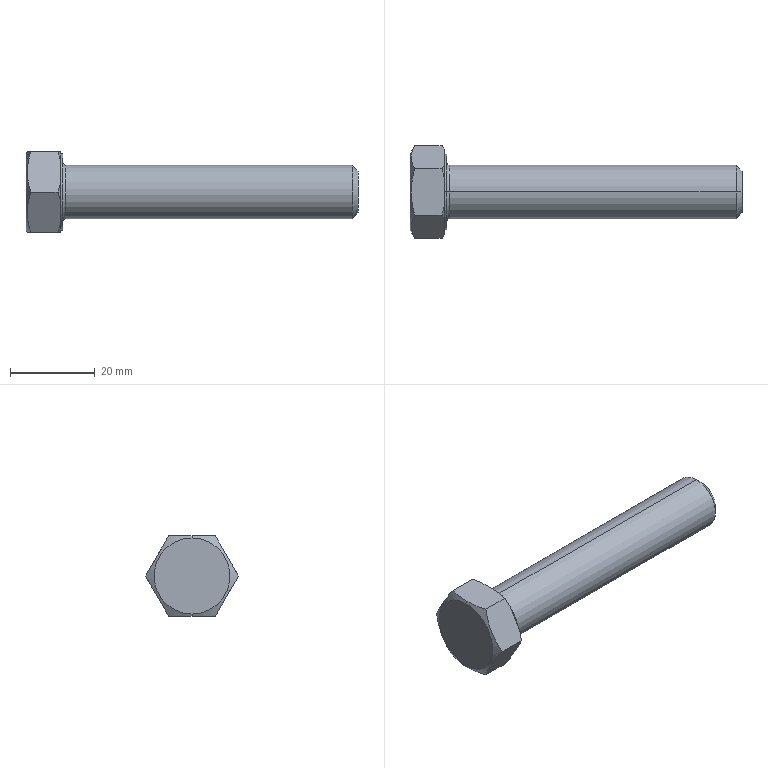Part | SolidWorks | features RevCut 4, Chamfer 1, Extrusion 1, Fillet 1, LPattern 1, Revolution 1 | 1 solid | 26 faces | box 78.581 x 21.997 x 19.05 mm | volume 11501 mm3 | cone 10 | plane 10 | cylinder 4 | torus 2 | commonest cylinder face diameters 12.7 x2 18 x2
STEP:
#1=CARTESIAN_POINT('',(9.331,0.,6.35));
#2=VERTEX_POINT('',#1);
#3=CARTESIAN_POINT('',(9.331,0.,-6.35));
#4=VERTEX_POINT('',#3);
#5=CARTESIAN_POINT('',(9.331,0.,0.));
#6=DIRECTION('',(1.,0.,0.));
#7=DIRECTION('',(0.,0.,-1.));
#8=AXIS2_PLACEMENT_3D('',#5,#6,#7);
#9=CIRCLE('',#8,6.35);
#10=EDGE_CURVE('',#2,#4,#9,.T.);
#11=ORIENTED_EDGE('',*,*,#10,.F.);
#12=CARTESIAN_POINT('',(8.731,0.,6.95));
#13=VERTEX_POINT('',#12);
#14=CARTESIAN_POINT('',(9.331,0.,6.95));
#15=DIRECTION('',(0.,1.,0.));
#16=DIRECTION('',(0.,0.,1.));
#17=AXIS2_PLACEMENT_3D('',#14,#15,#16);
#18=CIRCLE('',#17,0.6);
#19=EDGE_CURVE('',#2,#13,#18,.T.);
#20=ORIENTED_EDGE('',*,*,#19,.T.);
#21=CARTESIAN_POINT('',(8.731,0.,-6.95));
#22=VERTEX_POINT('',#21);
#23=CARTESIAN_POINT('',(8.731,0.,0.));
#24=DIRECTION('',(-1.,0.,0.));
#25=DIRECTION('',(0.,0.,-1.));
#26=AXIS2_PLACEMENT_3D('',#23,#24,#25);
#27=CIRCLE('',#26,6.95);
#28=EDGE_CURVE('',#22,#13,#27,.T.);
#29=ORIENTED_EDGE('',*,*,#28,.F.);
#30=CARTESIAN_POINT('',(9.331,0.,-6.95));
#31=DIRECTION('',(0.,-1.,0.));
#32=DIRECTION('',(0.,0.,-1.));
#33=AXIS2_PLACEMENT_3D('',#30,#31,#32);
#34=CIRCLE('',#33,0.6);
#35=EDGE_CURVE('',#4,#22,#34,.T.);
#36=ORIENTED_EDGE('',*,*,#35,.F.);
#37=EDGE_LOOP('',(#11,#20,#29,#36));
#38=FACE_OUTER_BOUND('',#37,.T.);
#39=CARTESIAN_POINT('',(9.331,0.,0.));
#40=DIRECTION('',(1.,0.,0.));
#41=DIRECTION('',(0.,0.,-1.));
#42=AXIS2_PLACEMENT_3D('',#39,#40,#41);
#43=TOROIDAL_SURFACE('',#42,6.95,0.6);
#44=ADVANCED_FACE('',(#38),#43,.F.);
#45=CARTESIAN_POINT('',(78.581,0.,-4.95));
#46=VERTEX_POINT('',#45);
#47=CARTESIAN_POINT('',(78.581,0.,4.95));
#48=VERTEX_POINT('',#47);
#49=CARTESIAN_POINT('',(78.581,0.,0.));
#50=DIRECTION('',(1.,0.,0.));
#51=DIRECTION('',(0.,0.,1.));
#52=AXIS2_PLACEMENT_3D('',#49,#50,#51);
#53=CIRCLE('',#52,4.95);
#54=EDGE_CURVE('',#46,#48,#53,.T.);
#55=ORIENTED_EDGE('',*,*,#54,.F.);
#56=CARTESIAN_POINT('',(77.181,0.,-6.35));
#57=VERTEX_POINT('',#56);
#58=CARTESIAN_POINT('',(77.181,0.,-6.35));
#59=DIRECTION('',(-0.7071,0.,-0.7071));
#60=VECTOR('',#59,1000.);
#61=LINE('',#58,#60);
#62=EDGE_CURVE('',#46,#57,#61,.T.);
#63=ORIENTED_EDGE('',*,*,#62,.T.);
#64=CARTESIAN_POINT('',(77.181,0.,6.35));
#65=VERTEX_POINT('',#64);
#66=CARTESIAN_POINT('',(77.181,0.,0.));
#67=DIRECTION('',(-1.,0.,0.));
#68=DIRECTION('',(0.,0.,1.));
#69=AXIS2_PLACEMENT_3D('',#66,#67,#68);
#70=CIRCLE('',#69,6.35);
#71=EDGE_CURVE('',#65,#57,#70,.T.);
#72=ORIENTED_EDGE('',*,*,#71,.F.);
#73=CARTESIAN_POINT('',(77.181,0.,6.35));
#74=DIRECTION('',(-0.7071,0.,0.7071));
#75=VECTOR('',#74,1000.);
#76=LINE('',#73,#75);
#77=EDGE_CURVE('',#48,#65,#76,.T.);
#78=ORIENTED_EDGE('',*,*,#77,.F.);
#79=EDGE_LOOP('',(#55,#63,#72,#78));
#80=FACE_OUTER_BOUND('',#79,.T.);
#81=CARTESIAN_POINT('',(77.181,0.,0.));
#82=DIRECTION('',(-1.,0.,0.));
#83=DIRECTION('',(0.,0.,1.));
#84=AXIS2_PLACEMENT_3D('',#81,#82,#83);
#85=CONICAL_SURFACE('',#84,6.35,0.7854);
#86=ADVANCED_FACE('',(#80),#85,.T.);
#87=ORIENTED_EDGE('',*,*,#71,.T.);
#88=CARTESIAN_POINT('',(0.,0.,-6.35));
#89=DIRECTION('',(-1.,0.,0.));
#90=VECTOR('',#89,1000.);
#91=LINE('',#88,#90);
#92=EDGE_CURVE('',#57,#4,#91,.T.);
#93=ORIENTED_EDGE('',*,*,#92,.T.);
#94=CARTESIAN_POINT('',(9.331,0.,0.));
#95=DIRECTION('',(1.,0.,0.));
#96=DIRECTION('',(0.,0.,-1.));
#97=AXIS2_PLACEMENT_3D('',#94,#95,#96);
#98=CIRCLE('',#97,6.35);
#99=EDGE_CURVE('',#4,#2,#98,.T.);
#100=ORIENTED_EDGE('',*,*,#99,.T.);
#101=CARTESIAN_POINT('',(0.,0.,6.35));
#102=DIRECTION('',(-1.,0.,0.));
#103=VECTOR('',#102,1000.);
#104=LINE('',#101,#103);
#105=EDGE_CURVE('',#65,#2,#104,.T.);
#106=ORIENTED_EDGE('',*,*,#105,.F.);
#107=EDGE_LOOP('',(#87,#93,#100,#106));
#108=FACE_OUTER_BOUND('',#107,.T.);
#109=CARTESIAN_POINT('',(0.,0.,0.));
#110=DIRECTION('',(-1.,0.,0.));
#111=DIRECTION('',(0.,0.,1.));
#112=AXIS2_PLACEMENT_3D('',#109,#110,#111);
#113=CYLINDRICAL_SURFACE('',#112,6.35);
#114=ADVANCED_FACE('',(#108),#113,.T.);
#115=CARTESIAN_POINT('',(8.731,0.,9.));
#116=VERTEX_POINT('',#115);
#117=CARTESIAN_POINT('',(8.731,0.,-9.));
#118=VERTEX_POINT('',#117);
#119=CARTESIAN_POINT('',(8.731,0.,0.));
#120=DIRECTION('',(-1.,0.,0.));
#121=DIRECTION('',(0.,0.,1.));
#122=AXIS2_PLACEMENT_3D('',#119,#120,#121);
#123=CIRCLE('',#122,9.);
#124=EDGE_CURVE('',#116,#118,#123,.T.);
#125=ORIENTED_EDGE('',*,*,#124,.T.);
#126=CARTESIAN_POINT('',(8.131,0.,-9.));
#127=VERTEX_POINT('',#126);
#128=CARTESIAN_POINT('',(0.,0.,-9.));
#129=DIRECTION('',(-1.,0.,0.));
#130=VECTOR('',#129,1000.);
#131=LINE('',#128,#130);
#132=EDGE_CURVE('',#118,#127,#131,.T.);
#133=ORIENTED_EDGE('',*,*,#132,.T.);
#134=CARTESIAN_POINT('',(8.131,0.,9.));
#135=VERTEX_POINT('',#134);
#136=CARTESIAN_POINT('',(8.131,0.,0.));
#137=DIRECTION('',(-1.,0.,0.));
#138=DIRECTION('',(0.,0.,1.));
#139=AXIS2_PLACEMENT_3D('',#136,#137,#138);
#140=CIRCLE('',#139,9.);
#141=EDGE_CURVE('',#135,#127,#140,.T.);
#142=ORIENTED_EDGE('',*,*,#141,.F.);
#143=CARTESIAN_POINT('',(0.,0.,9.));
#144=DIRECTION('',(-1.,0.,0.));
#145=VECTOR('',#144,1000.);
#146=LINE('',#143,#145);
#147=EDGE_CURVE('',#116,#135,#146,.T.);
#148=ORIENTED_EDGE('',*,*,#147,.F.);
#149=EDGE_LOOP('',(#125,#133,#142,#148));
#150=FACE_OUTER_BOUND('',#149,.T.);
#151=CARTESIAN_POINT('',(0.,0.,0.));
#152=DIRECTION('',(-1.,0.,0.));
#153=DIRECTION('',(0.,0.,1.));
#154=AXIS2_PLACEMENT_3D('',#151,#152,#153);
#155=CYLINDRICAL_SURFACE('',#154,9.);
#156=ADVANCED_FACE('',(#150),#155,.T.);
#157=CARTESIAN_POINT('',(0.,0.,9.));
#158=VERTEX_POINT('',#157);
#159=CARTESIAN_POINT('',(0.,0.,-9.));
#160=VERTEX_POINT('',#159);
#161=CARTESIAN_POINT('',(0.,0.,0.));
#162=DIRECTION('',(-1.,0.,0.));
#163=DIRECTION('',(0.,0.,1.));
#164=AXIS2_PLACEMENT_3D('',#161,#162,#163);
#165=CIRCLE('',#164,9.);
#166=EDGE_CURVE('',#158,#160,#165,.T.);
#167=ORIENTED_EDGE('',*,*,#166,.F.);
#168=CARTESIAN_POINT('',(0.3031,0.,9.525));
#169=VERTEX_POINT('',#168);
#170=CARTESIAN_POINT('',(0.,0.,9.));
#171=DIRECTION('',(0.5,0.,0.866));
#172=VECTOR('',#171,1000.);
#173=LINE('',#170,#172);
#174=EDGE_CURVE('',#158,#169,#173,.T.);
#175=ORIENTED_EDGE('',*,*,#174,.T.);
#176=CARTESIAN_POINT('',(1.154,5.499,9.525));
#177=VERTEX_POINT('',#176);
#178=CARTESIAN_POINT('',(0.3031,0.,9.525));
#179=CARTESIAN_POINT('',(0.3031,0.4656,9.525));
#180=CARTESIAN_POINT('',(0.323,0.9341,9.525));
#181=CARTESIAN_POINT('',(0.4017,1.87,9.525));
#182=CARTESIAN_POINT('',(0.4599,2.333,9.525));
#183=CARTESIAN_POINT('',(0.6834,3.709,9.525));
#184=CARTESIAN_POINT('',(0.8971,4.61,9.525));
#185=CARTESIAN_POINT('',(1.154,5.499,9.525));
#186=B_SPLINE_CURVE_WITH_KNOTS('',3,(#178,#179,#180,#181,#182,#183,#184,#185),.UNSPECIFIED.,.F.,.F.,(4,2,2,4),(0.01578,0.01717,0.01857,0.02135),.UNSPECIFIED.);
#187=EDGE_CURVE('',#169,#177,#186,.T.);
#188=ORIENTED_EDGE('',*,*,#187,.T.);
#189=CARTESIAN_POINT('',(1.154,10.999,0.));
#190=VERTEX_POINT('',#189);
#191=CARTESIAN_POINT('',(1.154,5.499,9.525));
#192=CARTESIAN_POINT('',(0.8946,5.948,8.747));
#193=CARTESIAN_POINT('',(0.681,6.4,7.964));
#194=CARTESIAN_POINT('',(0.3851,7.314,6.381));
#195=CARTESIAN_POINT('',(0.3037,7.776,5.581));
#196=CARTESIAN_POINT('',(0.3028,8.477,4.367));
#197=CARTESIAN_POINT('',(0.3227,8.712,3.96));
#198=CARTESIAN_POINT('',(0.4002,9.177,3.155));
#199=CARTESIAN_POINT('',(0.4578,9.408,2.756));
#200=CARTESIAN_POINT('',(0.6802,10.096,1.564));
#201=CARTESIAN_POINT('',(0.8943,10.549,0.7786));
#202=CARTESIAN_POINT('',(1.154,10.999,0.));
#203=B_SPLINE_CURVE_WITH_KNOTS('',3,(#191,#192,#193,#194,#195,#196,#197,#198,#199,#200,#201,#202),.UNSPECIFIED.,.F.,.F.,(4,2,2,2,2,4),(0.000000238,0.002777,0.005554,0.006943,0.008331,0.01111),.UNSPECIFIED.);
#204=EDGE_CURVE('',#177,#190,#203,.T.);
#205=ORIENTED_EDGE('',*,*,#204,.T.);
#206=CARTESIAN_POINT('',(1.154,5.499,-9.525));
#207=VERTEX_POINT('',#206);
#208=CARTESIAN_POINT('',(1.154,10.999,0.));
#209=CARTESIAN_POINT('',(0.8946,10.55,-0.7776));
#210=CARTESIAN_POINT('',(0.681,10.097,-1.561));
#211=CARTESIAN_POINT('',(0.3851,9.183,-3.144));
#212=CARTESIAN_POINT('',(0.3037,8.722,-3.944));
#213=CARTESIAN_POINT('',(0.3028,8.02,-5.158));
#214=CARTESIAN_POINT('',(0.3227,7.786,-5.565));
#215=CARTESIAN_POINT('',(0.4002,7.321,-6.37));
#216=CARTESIAN_POINT('',(0.4578,7.09,-6.769));
#217=CARTESIAN_POINT('',(0.6802,6.402,-7.961));
#218=CARTESIAN_POINT('',(0.8943,5.949,-8.746));
#219=CARTESIAN_POINT('',(1.154,5.499,-9.525));
#220=B_SPLINE_CURVE_WITH_KNOTS('',3,(#208,#209,#210,#211,#212,#213,#214,#215,#216,#217,#218,#219),.UNSPECIFIED.,.F.,.F.,(4,2,2,2,2,4),(0.000000238,0.002777,0.005554,0.006943,0.008331,0.01111),.UNSPECIFIED.);
#221=EDGE_CURVE('',#190,#207,#220,.T.);
#222=ORIENTED_EDGE('',*,*,#221,.T.);
#223=CARTESIAN_POINT('',(0.3031,0.,-9.525));
#224=VERTEX_POINT('',#223);
#225=CARTESIAN_POINT('',(1.154,5.499,-9.525));
#226=CARTESIAN_POINT('',(0.8971,4.61,-9.525));
#227=CARTESIAN_POINT('',(0.6834,3.709,-9.525));
#228=CARTESIAN_POINT('',(0.4599,2.333,-9.525));
#229=CARTESIAN_POINT('',(0.4017,1.87,-9.525));
#230=CARTESIAN_POINT('',(0.323,0.9341,-9.525));
#231=CARTESIAN_POINT('',(0.3031,0.4656,-9.525));
#232=CARTESIAN_POINT('',(0.3031,0.,-9.525));
#233=B_SPLINE_CURVE_WITH_KNOTS('',3,(#225,#226,#227,#228,#229,#230,#231,#232),.UNSPECIFIED.,.F.,.F.,(4,2,2,4),(0.02694,0.02972,0.03112,0.03251),.UNSPECIFIED.);
#234=EDGE_CURVE('',#207,#224,#233,.T.);
#235=ORIENTED_EDGE('',*,*,#234,.T.);
#236=CARTESIAN_POINT('',(0.,0.,-9.));
#237=DIRECTION('',(0.5,0.,-0.866));
#238=VECTOR('',#237,1000.);
#239=LINE('',#236,#238);
#240=EDGE_CURVE('',#160,#224,#239,.T.);
#241=ORIENTED_EDGE('',*,*,#240,.F.);
#242=EDGE_LOOP('',(#167,#175,#188,#205,#222,#235,#241));
#243=FACE_OUTER_BOUND('',#242,.T.);
#244=CARTESIAN_POINT('',(0.,0.,0.));
#245=DIRECTION('',(1.,0.,0.));
#246=DIRECTION('',(0.,0.,-1.));
#247=AXIS2_PLACEMENT_3D('',#244,#245,#246);
#248=CONICAL_SURFACE('',#247,9.,1.047);
#249=ADVANCED_FACE('',(#243),#248,.T.);
#250=CARTESIAN_POINT('',(8.131,6.663,-7.509));
#251=VERTEX_POINT('',#250);
#252=CARTESIAN_POINT('',(8.131,9.835,-2.016));
#253=VERTEX_POINT('',#252);
#254=CARTESIAN_POINT('',(8.131,5.499,-9.525));
#255=DIRECTION('',(0.,0.5,0.866));
#256=VECTOR('',#255,1000.);
#257=LINE('',#254,#256);
#258=EDGE_CURVE('',#251,#253,#257,.T.);
#259=ORIENTED_EDGE('',*,*,#258,.F.);
#260=CARTESIAN_POINT('',(7.577,5.499,-9.525));
#261=VERTEX_POINT('',#260);
#262=CARTESIAN_POINT('',(7.577,5.499,-9.525));
#263=CARTESIAN_POINT('',(7.8,5.884,-8.858));
#264=CARTESIAN_POINT('',(7.989,6.272,-8.186));
#265=CARTESIAN_POINT('',(8.131,6.663,-7.509));
#266=B_SPLINE_CURVE_WITH_KNOTS('',3,(#262,#263,#264,#265),.UNSPECIFIED.,.F.,.F.,(4,4),(0.000000238,0.002383),.UNSPECIFIED.);
#267=EDGE_CURVE('',#261,#251,#266,.T.);
#268=ORIENTED_EDGE('',*,*,#267,.F.);
#269=CARTESIAN_POINT('',(8.731,5.499,-9.525));
#270=DIRECTION('',(-1.,0.,0.));
#271=VECTOR('',#270,1000.);
#272=LINE('',#269,#271);
#273=EDGE_CURVE('',#261,#207,#272,.T.);
#274=ORIENTED_EDGE('',*,*,#273,.T.);
#275=ORIENTED_EDGE('',*,*,#221,.F.);
#276=CARTESIAN_POINT('',(7.577,10.999,0.));
#277=VERTEX_POINT('',#276);
#278=CARTESIAN_POINT('',(8.731,10.999,0.));
#279=DIRECTION('',(-1.,0.,0.));
#280=VECTOR('',#279,1000.);
#281=LINE('',#278,#280);
#282=EDGE_CURVE('',#277,#190,#281,.T.);
#283=ORIENTED_EDGE('',*,*,#282,.F.);
#284=CARTESIAN_POINT('',(8.131,9.835,-2.016));
#285=CARTESIAN_POINT('',(7.988,10.226,-1.338));
#286=CARTESIAN_POINT('',(7.8,10.614,-0.6665));
#287=CARTESIAN_POINT('',(7.577,10.999,0.));
#288=B_SPLINE_CURVE_WITH_KNOTS('',3,(#284,#285,#286,#287),.UNSPECIFIED.,.F.,.F.,(4,4),(0.008731,0.01111),.UNSPECIFIED.);
#289=EDGE_CURVE('',#253,#277,#288,.T.);
#290=ORIENTED_EDGE('',*,*,#289,.F.);
#291=EDGE_LOOP('',(#259,#268,#274,#275,#283,#290));
#292=FACE_OUTER_BOUND('',#291,.T.);
#293=CARTESIAN_POINT('',(8.731,5.499,-9.525));
#294=DIRECTION('',(0.,-0.866,0.5));
#295=DIRECTION('',(0.,-0.5,-0.866));
#296=AXIS2_PLACEMENT_3D('',#293,#294,#295);
#297=PLANE('',#296);
#298=ADVANCED_FACE('',(#292),#297,.F.);
#299=CARTESIAN_POINT('',(8.131,9.835,2.016));
#300=VERTEX_POINT('',#299);
#301=CARTESIAN_POINT('',(8.131,6.663,7.509));
#302=VERTEX_POINT('',#301);
#303=CARTESIAN_POINT('',(8.131,10.999,0.));
#304=DIRECTION('',(0.,-0.5,0.866));
#305=VECTOR('',#304,1000.);
#306=LINE('',#303,#305);
#307=EDGE_CURVE('',#300,#302,#306,.T.);
#308=ORIENTED_EDGE('',*,*,#307,.F.);
#309=CARTESIAN_POINT('',(7.577,10.999,0.));
#310=CARTESIAN_POINT('',(7.8,10.613,0.6672));
#311=CARTESIAN_POINT('',(7.989,10.226,1.339));
#312=CARTESIAN_POINT('',(8.131,9.835,2.016));
#313=B_SPLINE_CURVE_WITH_KNOTS('',3,(#309,#310,#311,#312),.UNSPECIFIED.,.F.,.F.,(4,4),(0.000000238,0.002383),.UNSPECIFIED.);
#314=EDGE_CURVE('',#277,#300,#313,.T.);
#315=ORIENTED_EDGE('',*,*,#314,.F.);
#316=ORIENTED_EDGE('',*,*,#282,.T.);
#317=ORIENTED_EDGE('',*,*,#204,.F.);
#318=CARTESIAN_POINT('',(7.577,5.499,9.525));
#319=VERTEX_POINT('',#318);
#320=CARTESIAN_POINT('',(8.731,5.499,9.525));
#321=DIRECTION('',(-1.,0.,0.));
#322=VECTOR('',#321,1000.);
#323=LINE('',#320,#322);
#324=EDGE_CURVE('',#319,#177,#323,.T.);
#325=ORIENTED_EDGE('',*,*,#324,.F.);
#326=CARTESIAN_POINT('',(8.131,6.663,7.509));
#327=CARTESIAN_POINT('',(7.988,6.272,8.187));
#328=CARTESIAN_POINT('',(7.8,5.884,8.859));
#329=CARTESIAN_POINT('',(7.577,5.499,9.525));
#330=B_SPLINE_CURVE_WITH_KNOTS('',3,(#326,#327,#328,#329),.UNSPECIFIED.,.F.,.F.,(4,4),(0.008731,0.01111),.UNSPECIFIED.);
#331=EDGE_CURVE('',#302,#319,#330,.T.);
#332=ORIENTED_EDGE('',*,*,#331,.F.);
#333=EDGE_LOOP('',(#308,#315,#316,#317,#325,#332));
#334=FACE_OUTER_BOUND('',#333,.T.);
#335=CARTESIAN_POINT('',(8.731,10.999,0.));
#336=DIRECTION('',(0.,-0.866,-0.5));
#337=DIRECTION('',(0.,0.5,-0.866));
#338=AXIS2_PLACEMENT_3D('',#335,#336,#337);
#339=PLANE('',#338);
#340=ADVANCED_FACE('',(#334),#339,.F.);
#341=CARTESIAN_POINT('',(8.131,3.172,9.525));
#342=VERTEX_POINT('',#341);
#343=CARTESIAN_POINT('',(8.131,-3.172,9.525));
#344=VERTEX_POINT('',#343);
#345=CARTESIAN_POINT('',(8.131,5.499,9.525));
#346=DIRECTION('',(0.,-1.,0.));
#347=VECTOR('',#346,1000.);
#348=LINE('',#345,#347);
#349=EDGE_CURVE('',#342,#344,#348,.T.);
#350=ORIENTED_EDGE('',*,*,#349,.F.);
#351=CARTESIAN_POINT('',(7.577,5.499,9.525));
#352=CARTESIAN_POINT('',(7.799,4.733,9.525));
#353=CARTESIAN_POINT('',(7.988,3.958,9.525));
#354=CARTESIAN_POINT('',(8.131,3.172,9.525));
#355=B_SPLINE_CURVE_WITH_KNOTS('',3,(#351,#352,#353,#354),.UNSPECIFIED.,.F.,.F.,(4,4),(0.02694,0.02934),.UNSPECIFIED.);
#356=EDGE_CURVE('',#319,#342,#355,.T.);
#357=ORIENTED_EDGE('',*,*,#356,.F.);
#358=ORIENTED_EDGE('',*,*,#324,.T.);
#359=ORIENTED_EDGE('',*,*,#187,.F.);
#360=CARTESIAN_POINT('',(1.154,-5.499,9.525));
#361=VERTEX_POINT('',#360);
#362=CARTESIAN_POINT('',(1.154,-5.499,9.525));
#363=CARTESIAN_POINT('',(0.8953,-4.604,9.525));
#364=CARTESIAN_POINT('',(0.679,-3.688,9.525));
#365=CARTESIAN_POINT('',(0.3832,-1.854,9.525));
#366=CARTESIAN_POINT('',(0.3031,-0.9305,9.525));
#367=CARTESIAN_POINT('',(0.3031,0.,9.525));
#368=B_SPLINE_CURVE_WITH_KNOTS('',3,(#362,#363,#364,#365,#366,#367),.UNSPECIFIED.,.F.,.F.,(4,2,4),(0.01021,0.013,0.01578),.UNSPECIFIED.);
#369=EDGE_CURVE('',#361,#169,#368,.T.);
#370=ORIENTED_EDGE('',*,*,#369,.F.);
#371=CARTESIAN_POINT('',(7.577,-5.499,9.525));
#372=VERTEX_POINT('',#371);
#373=CARTESIAN_POINT('',(8.731,-5.499,9.525));
#374=DIRECTION('',(-1.,0.,0.));
#375=VECTOR('',#374,1000.);
#376=LINE('',#373,#375);
#377=EDGE_CURVE('',#372,#361,#376,.T.);
#378=ORIENTED_EDGE('',*,*,#377,.F.);
#379=CARTESIAN_POINT('',(8.131,-3.172,9.525));
#380=CARTESIAN_POINT('',(7.989,-3.954,9.525));
#381=CARTESIAN_POINT('',(7.798,-4.734,9.525));
#382=CARTESIAN_POINT('',(7.577,-5.499,9.525));
#383=B_SPLINE_CURVE_WITH_KNOTS('',3,(#379,#380,#381,#382),.UNSPECIFIED.,.F.,.F.,(4,4),(0.0357,0.03808),.UNSPECIFIED.);
#384=EDGE_CURVE('',#344,#372,#383,.T.);
#385=ORIENTED_EDGE('',*,*,#384,.F.);
#386=EDGE_LOOP('',(#350,#357,#358,#359,#370,#378,#385));
#387=FACE_OUTER_BOUND('',#386,.T.);
#388=CARTESIAN_POINT('',(8.731,5.499,9.525));
#389=DIRECTION('',(0.,0.,-1.));
#390=DIRECTION('',(-1.,0.,0.));
#391=AXIS2_PLACEMENT_3D('',#388,#389,#390);
#392=PLANE('',#391);
#393=ADVANCED_FACE('',(#387),#392,.F.);
#394=CARTESIAN_POINT('',(8.131,-6.663,7.509));
#395=VERTEX_POINT('',#394);
#396=CARTESIAN_POINT('',(8.131,-9.835,2.016));
#397=VERTEX_POINT('',#396);
#398=CARTESIAN_POINT('',(8.131,-10.999,0.));
#399=DIRECTION('',(0.,-0.5,-0.866));
#400=VECTOR('',#399,1000.);
#401=LINE('',#398,#400);
#402=EDGE_CURVE('',#395,#397,#401,.T.);
#403=ORIENTED_EDGE('',*,*,#402,.F.);
#404=CARTESIAN_POINT('',(7.577,-5.499,9.525));
#405=CARTESIAN_POINT('',(7.8,-5.884,8.858));
#406=CARTESIAN_POINT('',(7.989,-6.272,8.186));
#407=CARTESIAN_POINT('',(8.131,-6.663,7.509));
#408=B_SPLINE_CURVE_WITH_KNOTS('',3,(#404,#405,#406,#407),.UNSPECIFIED.,.F.,.F.,(4,4),(0.000000238,0.002383),.UNSPECIFIED.);
#409=EDGE_CURVE('',#372,#395,#408,.T.);
#410=ORIENTED_EDGE('',*,*,#409,.F.);
#411=ORIENTED_EDGE('',*,*,#377,.T.);
#412=CARTESIAN_POINT('',(1.154,-10.999,0.));
#413=VERTEX_POINT('',#412);
#414=CARTESIAN_POINT('',(1.154,-10.999,0.));
#415=CARTESIAN_POINT('',(0.8946,-10.55,0.7776));
#416=CARTESIAN_POINT('',(0.681,-10.097,1.561));
#417=CARTESIAN_POINT('',(0.3851,-9.183,3.144));
#418=CARTESIAN_POINT('',(0.3037,-8.722,3.944));
#419=CARTESIAN_POINT('',(0.3028,-8.02,5.158));
#420=CARTESIAN_POINT('',(0.3227,-7.786,5.565));
#421=CARTESIAN_POINT('',(0.4002,-7.321,6.37));
#422=CARTESIAN_POINT('',(0.4578,-7.09,6.769));
#423=CARTESIAN_POINT('',(0.6802,-6.402,7.961));
#424=CARTESIAN_POINT('',(0.8943,-5.949,8.746));
#425=CARTESIAN_POINT('',(1.154,-5.499,9.525));
#426=B_SPLINE_CURVE_WITH_KNOTS('',3,(#414,#415,#416,#417,#418,#419,#420,#421,#422,#423,#424,#425),.UNSPECIFIED.,.F.,.F.,(4,2,2,2,2,4),(0.000000238,0.002777,0.005554,0.006943,0.008331,0.01111),.UNSPECIFIED.);
#427=EDGE_CURVE('',#413,#361,#426,.T.);
#428=ORIENTED_EDGE('',*,*,#427,.F.);
#429=CARTESIAN_POINT('',(7.577,-10.999,0.));
#430=VERTEX_POINT('',#429);
#431=CARTESIAN_POINT('',(8.731,-10.999,0.));
#432=DIRECTION('',(-1.,0.,0.));
#433=VECTOR('',#432,1000.);
#434=LINE('',#431,#433);
#435=EDGE_CURVE('',#430,#413,#434,.T.);
#436=ORIENTED_EDGE('',*,*,#435,.F.);
#437=CARTESIAN_POINT('',(8.131,-9.835,2.016));
#438=CARTESIAN_POINT('',(7.988,-10.226,1.338));
#439=CARTESIAN_POINT('',(7.8,-10.614,0.6665));
#440=CARTESIAN_POINT('',(7.577,-10.999,0.));
#441=B_SPLINE_CURVE_WITH_KNOTS('',3,(#437,#438,#439,#440),.UNSPECIFIED.,.F.,.F.,(4,4),(0.008731,0.01111),.UNSPECIFIED.);
#442=EDGE_CURVE('',#397,#430,#441,.T.);
#443=ORIENTED_EDGE('',*,*,#442,.F.);
#444=EDGE_LOOP('',(#403,#410,#411,#428,#436,#443));
#445=FACE_OUTER_BOUND('',#444,.T.);
#446=CARTESIAN_POINT('',(8.731,-10.999,0.));
#447=DIRECTION('',(0.,0.866,-0.5));
#448=DIRECTION('',(0.,0.5,0.866));
#449=AXIS2_PLACEMENT_3D('',#446,#447,#448);
#450=PLANE('',#449);
#451=ADVANCED_FACE('',(#445),#450,.F.);
#452=CARTESIAN_POINT('',(8.131,-9.835,-2.016));
#453=VERTEX_POINT('',#452);
#454=CARTESIAN_POINT('',(8.131,-6.663,-7.509));
#455=VERTEX_POINT('',#454);
#456=CARTESIAN_POINT('',(8.131,-5.499,-9.525));
#457=DIRECTION('',(0.,0.5,-0.866));
#458=VECTOR('',#457,1000.);
#459=LINE('',#456,#458);
#460=EDGE_CURVE('',#453,#455,#459,.T.);
#461=ORIENTED_EDGE('',*,*,#460,.F.);
#462=CARTESIAN_POINT('',(7.577,-10.999,0.));
#463=CARTESIAN_POINT('',(7.8,-10.613,-0.6672));
#464=CARTESIAN_POINT('',(7.989,-10.226,-1.339));
#465=CARTESIAN_POINT('',(8.131,-9.835,-2.016));
#466=B_SPLINE_CURVE_WITH_KNOTS('',3,(#462,#463,#464,#465),.UNSPECIFIED.,.F.,.F.,(4,4),(0.000000238,0.002383),.UNSPECIFIED.);
#467=EDGE_CURVE('',#430,#453,#466,.T.);
#468=ORIENTED_EDGE('',*,*,#467,.F.);
#469=ORIENTED_EDGE('',*,*,#435,.T.);
#470=CARTESIAN_POINT('',(1.154,-5.499,-9.525));
#471=VERTEX_POINT('',#470);
#472=CARTESIAN_POINT('',(1.154,-5.499,-9.525));
#473=CARTESIAN_POINT('',(0.8946,-5.948,-8.747));
#474=CARTESIAN_POINT('',(0.681,-6.4,-7.964));
#475=CARTESIAN_POINT('',(0.3851,-7.314,-6.381));
#476=CARTESIAN_POINT('',(0.3037,-7.776,-5.581));
#477=CARTESIAN_POINT('',(0.3028,-8.477,-4.367));
#478=CARTESIAN_POINT('',(0.3227,-8.712,-3.96));
#479=CARTESIAN_POINT('',(0.4002,-9.177,-3.155));
#480=CARTESIAN_POINT('',(0.4578,-9.408,-2.756));
#481=CARTESIAN_POINT('',(0.6802,-10.096,-1.564));
#482=CARTESIAN_POINT('',(0.8943,-10.549,-0.7786));
#483=CARTESIAN_POINT('',(1.154,-10.999,0.));
#484=B_SPLINE_CURVE_WITH_KNOTS('',3,(#472,#473,#474,#475,#476,#477,#478,#479,#480,#481,#482,#483),.UNSPECIFIED.,.F.,.F.,(4,2,2,2,2,4),(0.000000238,0.002777,0.005554,0.006943,0.008331,0.01111),.UNSPECIFIED.);
#485=EDGE_CURVE('',#471,#413,#484,.T.);
#486=ORIENTED_EDGE('',*,*,#485,.F.);
#487=CARTESIAN_POINT('',(7.577,-5.499,-9.525));
#488=VERTEX_POINT('',#487);
#489=CARTESIAN_POINT('',(8.731,-5.499,-9.525));
#490=DIRECTION('',(-1.,0.,0.));
#491=VECTOR('',#490,1000.);
#492=LINE('',#489,#491);
#493=EDGE_CURVE('',#488,#471,#492,.T.);
#494=ORIENTED_EDGE('',*,*,#493,.F.);
#495=CARTESIAN_POINT('',(8.131,-6.663,-7.509));
#496=CARTESIAN_POINT('',(7.988,-6.272,-8.187));
#497=CARTESIAN_POINT('',(7.8,-5.884,-8.859));
#498=CARTESIAN_POINT('',(7.577,-5.499,-9.525));
#499=B_SPLINE_CURVE_WITH_KNOTS('',3,(#495,#496,#497,#498),.UNSPECIFIED.,.F.,.F.,(4,4),(0.008731,0.01111),.UNSPECIFIED.);
#500=EDGE_CURVE('',#455,#488,#499,.T.);
#501=ORIENTED_EDGE('',*,*,#500,.F.);
#502=EDGE_LOOP('',(#461,#468,#469,#486,#494,#501));
#503=FACE_OUTER_BOUND('',#502,.T.);
#504=CARTESIAN_POINT('',(8.731,-5.499,-9.525));
#505=DIRECTION('',(0.,0.866,0.5));
#506=DIRECTION('',(0.,-0.5,0.866));
#507=AXIS2_PLACEMENT_3D('',#504,#505,#506);
#508=PLANE('',#507);
#509=ADVANCED_FACE('',(#503),#508,.F.);
#510=CARTESIAN_POINT('',(8.131,-3.172,-9.525));
#511=VERTEX_POINT('',#510);
#512=CARTESIAN_POINT('',(8.131,3.172,-9.525));
#513=VERTEX_POINT('',#512);
#514=CARTESIAN_POINT('',(8.131,5.499,-9.525));
#515=DIRECTION('',(0.,1.,0.));
#516=VECTOR('',#515,1000.);
#517=LINE('',#514,#516);
#518=EDGE_CURVE('',#511,#513,#517,.T.);
#519=ORIENTED_EDGE('',*,*,#518,.F.);
#520=CARTESIAN_POINT('',(7.577,-5.499,-9.525));
#521=CARTESIAN_POINT('',(7.798,-4.734,-9.525));
#522=CARTESIAN_POINT('',(7.989,-3.954,-9.525));
#523=CARTESIAN_POINT('',(8.131,-3.172,-9.525));
#524=B_SPLINE_CURVE_WITH_KNOTS('',3,(#520,#521,#522,#523),.UNSPECIFIED.,.F.,.F.,(4,4),(0.01021,0.01259),.UNSPECIFIED.);
#525=EDGE_CURVE('',#488,#511,#524,.T.);
#526=ORIENTED_EDGE('',*,*,#525,.F.);
#527=ORIENTED_EDGE('',*,*,#493,.T.);
#528=CARTESIAN_POINT('',(0.3031,0.,-9.525));
#529=CARTESIAN_POINT('',(0.3031,-0.9305,-9.525));
#530=CARTESIAN_POINT('',(0.3832,-1.854,-9.525));
#531=CARTESIAN_POINT('',(0.679,-3.688,-9.525));
#532=CARTESIAN_POINT('',(0.8953,-4.604,-9.525));
#533=CARTESIAN_POINT('',(1.154,-5.499,-9.525));
#534=B_SPLINE_CURVE_WITH_KNOTS('',3,(#528,#529,#530,#531,#532,#533),.UNSPECIFIED.,.F.,.F.,(4,2,4),(0.03251,0.03529,0.03808),.UNSPECIFIED.);
#535=EDGE_CURVE('',#224,#471,#534,.T.);
#536=ORIENTED_EDGE('',*,*,#535,.F.);
#537=ORIENTED_EDGE('',*,*,#234,.F.);
#538=ORIENTED_EDGE('',*,*,#273,.F.);
#539=CARTESIAN_POINT('',(8.131,3.172,-9.525));
#540=CARTESIAN_POINT('',(7.988,3.958,-9.525));
#541=CARTESIAN_POINT('',(7.799,4.733,-9.525));
#542=CARTESIAN_POINT('',(7.577,5.499,-9.525));
#543=B_SPLINE_CURVE_WITH_KNOTS('',3,(#539,#540,#541,#542),.UNSPECIFIED.,.F.,.F.,(4,4),(0.01895,0.02135),.UNSPECIFIED.);
#544=EDGE_CURVE('',#513,#261,#543,.T.);
#545=ORIENTED_EDGE('',*,*,#544,.F.);
#546=EDGE_LOOP('',(#519,#526,#527,#536,#537,#538,#545));
#547=FACE_OUTER_BOUND('',#546,.T.);
#548=CARTESIAN_POINT('',(8.731,5.499,-9.525));
#549=DIRECTION('',(0.,0.,1.));
#550=DIRECTION('',(1.,0.,0.));
#551=AXIS2_PLACEMENT_3D('',#548,#549,#550);
#552=PLANE('',#551);
#553=ADVANCED_FACE('',(#547),#552,.F.);
#554=ORIENTED_EDGE('',*,*,#525,.T.);
#555=CARTESIAN_POINT('',(8.131,0.,0.));
#556=DIRECTION('',(-1.,0.,0.));
#557=DIRECTION('',(0.,0.,-1.));
#558=AXIS2_PLACEMENT_3D('',#555,#556,#557);
#559=CIRCLE('',#558,10.039);
#560=EDGE_CURVE('',#511,#455,#559,.T.);
#561=ORIENTED_EDGE('',*,*,#560,.T.);
#562=ORIENTED_EDGE('',*,*,#500,.T.);
#563=EDGE_LOOP('',(#554,#561,#562));
#564=FACE_OUTER_BOUND('',#563,.T.);
#565=CARTESIAN_POINT('',(4.691,0.,0.));
#566=DIRECTION('',(-1.,0.,0.));
#567=DIRECTION('',(0.,0.,1.));
#568=AXIS2_PLACEMENT_3D('',#565,#566,#567);
#569=CONICAL_SURFACE('',#568,15.999,1.047);
#570=ADVANCED_FACE('',(#564),#569,.T.);
#571=ORIENTED_EDGE('',*,*,#467,.T.);
#572=CARTESIAN_POINT('',(8.131,0.,0.));
#573=DIRECTION('',(-1.,0.,0.));
#574=DIRECTION('',(0.,0.,-1.));
#575=AXIS2_PLACEMENT_3D('',#572,#573,#574);
#576=CIRCLE('',#575,10.039);
#577=EDGE_CURVE('',#453,#397,#576,.T.);
#578=ORIENTED_EDGE('',*,*,#577,.T.);
#579=ORIENTED_EDGE('',*,*,#442,.T.);
#580=EDGE_LOOP('',(#571,#578,#579));
#581=FACE_OUTER_BOUND('',#580,.T.);
#582=CARTESIAN_POINT('',(4.691,0.,0.));
#583=DIRECTION('',(-1.,0.,0.));
#584=DIRECTION('',(0.,0.,1.));
#585=AXIS2_PLACEMENT_3D('',#582,#583,#584);
#586=CONICAL_SURFACE('',#585,15.999,1.047);
#587=ADVANCED_FACE('',(#581),#586,.T.);
#588=ORIENTED_EDGE('',*,*,#409,.T.);
#589=CARTESIAN_POINT('',(8.131,0.,0.));
#590=DIRECTION('',(-1.,0.,0.));
#591=DIRECTION('',(0.,0.,-1.));
#592=AXIS2_PLACEMENT_3D('',#589,#590,#591);
#593=CIRCLE('',#592,10.039);
#594=EDGE_CURVE('',#395,#344,#593,.T.);
#595=ORIENTED_EDGE('',*,*,#594,.T.);
#596=ORIENTED_EDGE('',*,*,#384,.T.);
#597=EDGE_LOOP('',(#588,#595,#596));
#598=FACE_OUTER_BOUND('',#597,.T.);
#599=CARTESIAN_POINT('',(4.691,0.,0.));
#600=DIRECTION('',(-1.,0.,0.));
#601=DIRECTION('',(0.,0.,1.));
#602=AXIS2_PLACEMENT_3D('',#599,#600,#601);
#603=CONICAL_SURFACE('',#602,15.999,1.047);
#604=ADVANCED_FACE('',(#598),#603,.T.);
#605=ORIENTED_EDGE('',*,*,#356,.T.);
#606=CARTESIAN_POINT('',(8.131,0.,0.));
#607=DIRECTION('',(-1.,0.,0.));
#608=DIRECTION('',(0.,0.,-1.));
#609=AXIS2_PLACEMENT_3D('',#606,#607,#608);
#610=CIRCLE('',#609,10.039);
#611=EDGE_CURVE('',#342,#302,#610,.T.);
#612=ORIENTED_EDGE('',*,*,#611,.T.);
#613=ORIENTED_EDGE('',*,*,#331,.T.);
#614=EDGE_LOOP('',(#605,#612,#613));
#615=FACE_OUTER_BOUND('',#614,.T.);
#616=CARTESIAN_POINT('',(4.691,0.,0.));
#617=DIRECTION('',(-1.,0.,0.));
#618=DIRECTION('',(0.,0.,1.));
#619=AXIS2_PLACEMENT_3D('',#616,#617,#618);
#620=CONICAL_SURFACE('',#619,15.999,1.047);
#621=ADVANCED_FACE('',(#615),#620,.T.);
#622=ORIENTED_EDGE('',*,*,#314,.T.);
#623=CARTESIAN_POINT('',(8.131,0.,0.));
#624=DIRECTION('',(-1.,0.,0.));
#625=DIRECTION('',(0.,0.,-1.));
#626=AXIS2_PLACEMENT_3D('',#623,#624,#625);
#627=CIRCLE('',#626,10.039);
#628=EDGE_CURVE('',#300,#253,#627,.T.);
#629=ORIENTED_EDGE('',*,*,#628,.T.);
#630=ORIENTED_EDGE('',*,*,#289,.T.);
#631=EDGE_LOOP('',(#622,#629,#630));
#632=FACE_OUTER_BOUND('',#631,.T.);
#633=CARTESIAN_POINT('',(4.691,0.,0.));
#634=DIRECTION('',(-1.,0.,0.));
#635=DIRECTION('',(0.,0.,1.));
#636=AXIS2_PLACEMENT_3D('',#633,#634,#635);
#637=CONICAL_SURFACE('',#636,15.999,1.047);
#638=ADVANCED_FACE('',(#632),#637,.T.);
#639=ORIENTED_EDGE('',*,*,#267,.T.);
#640=CARTESIAN_POINT('',(8.131,0.,0.));
#641=DIRECTION('',(-1.,0.,0.));
#642=DIRECTION('',(0.,0.,-1.));
#643=AXIS2_PLACEMENT_3D('',#640,#641,#642);
#644=CIRCLE('',#643,10.039);
#645=EDGE_CURVE('',#251,#513,#644,.T.);
#646=ORIENTED_EDGE('',*,*,#645,.T.);
#647=ORIENTED_EDGE('',*,*,#544,.T.);
#648=EDGE_LOOP('',(#639,#646,#647));
#649=FACE_OUTER_BOUND('',#648,.T.);
#650=CARTESIAN_POINT('',(4.691,0.,0.));
#651=DIRECTION('',(-1.,0.,0.));
#652=DIRECTION('',(0.,0.,1.));
#653=AXIS2_PLACEMENT_3D('',#650,#651,#652);
#654=CONICAL_SURFACE('',#653,15.999,1.047);
#655=ADVANCED_FACE('',(#649),#654,.T.);
#656=ORIENTED_EDGE('',*,*,#174,.F.);
#657=CARTESIAN_POINT('',(0.,0.,0.));
#658=DIRECTION('',(-1.,0.,0.));
#659=DIRECTION('',(0.,0.,1.));
#660=AXIS2_PLACEMENT_3D('',#657,#658,#659);
#661=CIRCLE('',#660,9.);
#662=EDGE_CURVE('',#160,#158,#661,.T.);
#663=ORIENTED_EDGE('',*,*,#662,.F.);
#664=ORIENTED_EDGE('',*,*,#240,.T.);
#665=ORIENTED_EDGE('',*,*,#535,.T.);
#666=ORIENTED_EDGE('',*,*,#485,.T.);
#667=ORIENTED_EDGE('',*,*,#427,.T.);
#668=ORIENTED_EDGE('',*,*,#369,.T.);
#669=EDGE_LOOP('',(#656,#663,#664,#665,#666,#667,#668));
#670=FACE_OUTER_BOUND('',#669,.T.);
#671=CARTESIAN_POINT('',(0.,0.,0.));
#672=DIRECTION('',(1.,0.,0.));
#673=DIRECTION('',(0.,0.,-1.));
#674=AXIS2_PLACEMENT_3D('',#671,#672,#673);
#675=CONICAL_SURFACE('',#674,9.,1.047);
#676=ADVANCED_FACE('',(#670),#675,.T.);
#677=ORIENTED_EDGE('',*,*,#662,.T.);
#678=ORIENTED_EDGE('',*,*,#166,.T.);
#679=EDGE_LOOP('',(#677,#678));
#680=FACE_OUTER_BOUND('',#679,.T.);
#681=CARTESIAN_POINT('',(0.,10.999,0.));
#682=DIRECTION('',(1.,0.,0.));
#683=DIRECTION('',(0.,0.,-1.));
#684=AXIS2_PLACEMENT_3D('',#681,#682,#683);
#685=PLANE('',#684);
#686=ADVANCED_FACE('',(#680),#685,.F.);
#687=ORIENTED_EDGE('',*,*,#402,.T.);
#688=ORIENTED_EDGE('',*,*,#577,.F.);
#689=ORIENTED_EDGE('',*,*,#460,.T.);
#690=ORIENTED_EDGE('',*,*,#560,.F.);
#691=ORIENTED_EDGE('',*,*,#518,.T.);
#692=ORIENTED_EDGE('',*,*,#645,.F.);
#693=ORIENTED_EDGE('',*,*,#258,.T.);
#694=ORIENTED_EDGE('',*,*,#628,.F.);
#695=ORIENTED_EDGE('',*,*,#307,.T.);
#696=ORIENTED_EDGE('',*,*,#611,.F.);
#697=ORIENTED_EDGE('',*,*,#349,.T.);
#698=ORIENTED_EDGE('',*,*,#594,.F.);
#699=EDGE_LOOP('',(#687,#688,#689,#690,#691,#692,#693,#694,#695,#696,#697,#698));
#700=FACE_OUTER_BOUND('',#699,.T.);
#701=ORIENTED_EDGE('',*,*,#141,.T.);
#702=CARTESIAN_POINT('',(8.131,0.,0.));
#703=DIRECTION('',(-1.,0.,0.));
#704=DIRECTION('',(0.,0.,1.));
#705=AXIS2_PLACEMENT_3D('',#702,#703,#704);
#706=CIRCLE('',#705,9.);
#707=EDGE_CURVE('',#127,#135,#706,.T.);
#708=ORIENTED_EDGE('',*,*,#707,.T.);
#709=EDGE_LOOP('',(#701,#708));
#710=FACE_BOUND('',#709,.T.);
#711=CARTESIAN_POINT('',(8.131,9.,0.));
#712=DIRECTION('',(1.,0.,0.));
#713=DIRECTION('',(0.,0.,-1.));
#714=AXIS2_PLACEMENT_3D('',#711,#712,#713);
#715=PLANE('',#714);
#716=ADVANCED_FACE('',(#700,#710),#715,.T.);
#717=ORIENTED_EDGE('',*,*,#132,.F.);
#718=CARTESIAN_POINT('',(8.731,0.,0.));
#719=DIRECTION('',(-1.,0.,0.));
#720=DIRECTION('',(0.,0.,1.));
#721=AXIS2_PLACEMENT_3D('',#718,#719,#720);
#722=CIRCLE('',#721,9.);
#723=EDGE_CURVE('',#118,#116,#722,.T.);
#724=ORIENTED_EDGE('',*,*,#723,.T.);
#725=ORIENTED_EDGE('',*,*,#147,.T.);
#726=ORIENTED_EDGE('',*,*,#707,.F.);
#727=EDGE_LOOP('',(#717,#724,#725,#726));
#728=FACE_OUTER_BOUND('',#727,.T.);
#729=CARTESIAN_POINT('',(0.,0.,0.));
#730=DIRECTION('',(-1.,0.,0.));
#731=DIRECTION('',(0.,0.,1.));
#732=AXIS2_PLACEMENT_3D('',#729,#730,#731);
#733=CYLINDRICAL_SURFACE('',#732,9.);
#734=ADVANCED_FACE('',(#728),#733,.T.);
#735=CARTESIAN_POINT('',(78.581,0.,0.));
#736=DIRECTION('',(1.,0.,0.));
#737=DIRECTION('',(0.,0.,1.));
#738=AXIS2_PLACEMENT_3D('',#735,#736,#737);
#739=CIRCLE('',#738,4.95);
#740=EDGE_CURVE('',#48,#46,#739,.T.);
#741=ORIENTED_EDGE('',*,*,#740,.T.);
#742=ORIENTED_EDGE('',*,*,#54,.T.);
#743=EDGE_LOOP('',(#741,#742));
#744=FACE_OUTER_BOUND('',#743,.T.);
#745=CARTESIAN_POINT('',(78.581,0.,0.));
#746=DIRECTION('',(-1.,0.,0.));
#747=DIRECTION('',(0.,0.,1.));
#748=AXIS2_PLACEMENT_3D('',#745,#746,#747);
#749=PLANE('',#748);
#750=ADVANCED_FACE('',(#744),#749,.F.);
#751=ORIENTED_EDGE('',*,*,#92,.F.);
#752=CARTESIAN_POINT('',(77.181,0.,0.));
#753=DIRECTION('',(-1.,0.,0.));
#754=DIRECTION('',(0.,0.,1.));
#755=AXIS2_PLACEMENT_3D('',#752,#753,#754);
#756=CIRCLE('',#755,6.35);
#757=EDGE_CURVE('',#57,#65,#756,.T.);
#758=ORIENTED_EDGE('',*,*,#757,.T.);
#759=ORIENTED_EDGE('',*,*,#105,.T.);
#760=ORIENTED_EDGE('',*,*,#10,.T.);
#761=EDGE_LOOP('',(#751,#758,#759,#760));
#762=FACE_OUTER_BOUND('',#761,.T.);
#763=CARTESIAN_POINT('',(0.,0.,0.));
#764=DIRECTION('',(-1.,0.,0.));
#765=DIRECTION('',(0.,0.,1.));
#766=AXIS2_PLACEMENT_3D('',#763,#764,#765);
#767=CYLINDRICAL_SURFACE('',#766,6.35);
#768=ADVANCED_FACE('',(#762),#767,.T.);
#769=ORIENTED_EDGE('',*,*,#28,.T.);
#770=CARTESIAN_POINT('',(8.731,0.,0.));
#771=DIRECTION('',(-1.,0.,0.));
#772=DIRECTION('',(0.,0.,-1.));
#773=AXIS2_PLACEMENT_3D('',#770,#771,#772);
#774=CIRCLE('',#773,6.95);
#775=EDGE_CURVE('',#13,#22,#774,.T.);
#776=ORIENTED_EDGE('',*,*,#775,.T.);
#777=EDGE_LOOP('',(#769,#776));
#778=FACE_BOUND('',#777,.T.);
#779=ORIENTED_EDGE('',*,*,#124,.F.);
#780=ORIENTED_EDGE('',*,*,#723,.F.);
#781=EDGE_LOOP('',(#779,#780));
#782=FACE_OUTER_BOUND('',#781,.T.);
#783=CARTESIAN_POINT('',(8.731,10.999,0.));
#784=DIRECTION('',(1.,0.,0.));
#785=DIRECTION('',(0.,0.,-1.));
#786=AXIS2_PLACEMENT_3D('',#783,#784,#785);
#787=PLANE('',#786);
#788=ADVANCED_FACE('',(#778,#782),#787,.T.);
#789=ORIENTED_EDGE('',*,*,#62,.F.);
#790=ORIENTED_EDGE('',*,*,#740,.F.);
#791=ORIENTED_EDGE('',*,*,#77,.T.);
#792=ORIENTED_EDGE('',*,*,#757,.F.);
#793=EDGE_LOOP('',(#789,#790,#791,#792));
#794=FACE_OUTER_BOUND('',#793,.T.);
#795=CARTESIAN_POINT('',(77.181,0.,0.));
#796=DIRECTION('',(-1.,0.,0.));
#797=DIRECTION('',(0.,0.,1.));
#798=AXIS2_PLACEMENT_3D('',#795,#796,#797);
#799=CONICAL_SURFACE('',#798,6.35,0.7854);
#800=ADVANCED_FACE('',(#794),#799,.T.);
#801=ORIENTED_EDGE('',*,*,#19,.F.);
#802=ORIENTED_EDGE('',*,*,#99,.F.);
#803=ORIENTED_EDGE('',*,*,#35,.T.);
#804=ORIENTED_EDGE('',*,*,#775,.F.);
#805=EDGE_LOOP('',(#801,#802,#803,#804));
#806=FACE_OUTER_BOUND('',#805,.T.);
#807=CARTESIAN_POINT('',(9.331,0.,0.));
#808=DIRECTION('',(1.,0.,0.));
#809=DIRECTION('',(0.,0.,-1.));
#810=AXIS2_PLACEMENT_3D('',#807,#808,#809);
#811=TOROIDAL_SURFACE('',#810,6.95,0.6);
#812=ADVANCED_FACE('',(#806),#811,.F.);
#813=CLOSED_SHELL('',(#44,#86,#114,#156,#249,#298,#340,#393,#451,#509,#553,#570,#587,#604,#621,#638,#655,#676,#686,#716,#734,#750,#768,#788,#800,#812));
#814=MANIFOLD_SOLID_BREP('',#813);
#815=CARTESIAN_POINT('',(0.,0.,0.));
#816=DIRECTION('',(0.,0.,1.));
#817=DIRECTION('',(1.,0.,0.));
#818=AXIS2_PLACEMENT_3D('',#815,#816,#817);
#819=(LENGTH_UNIT()NAMED_UNIT(*)SI_UNIT(.MILLI.,.METRE.));
#820=UNCERTAINTY_MEASURE_WITH_UNIT(LENGTH_MEASURE(0.00001),#819,'','');
#821=(NAMED_UNIT(*)PLANE_ANGLE_UNIT()SI_UNIT($,.RADIAN.));
#822=(NAMED_UNIT(*)SI_UNIT($,.STERADIAN.)SOLID_ANGLE_UNIT());
#823=(GEOMETRIC_REPRESENTATION_CONTEXT(3)GLOBAL_UNCERTAINTY_ASSIGNED_CONTEXT((#820))GLOBAL_UNIT_ASSIGNED_CONTEXT((#819,#821,#822))REPRESENTATION_CONTEXT('',''));
#824=ADVANCED_BREP_SHAPE_REPRESENTATION('',(#814,#818),#823);